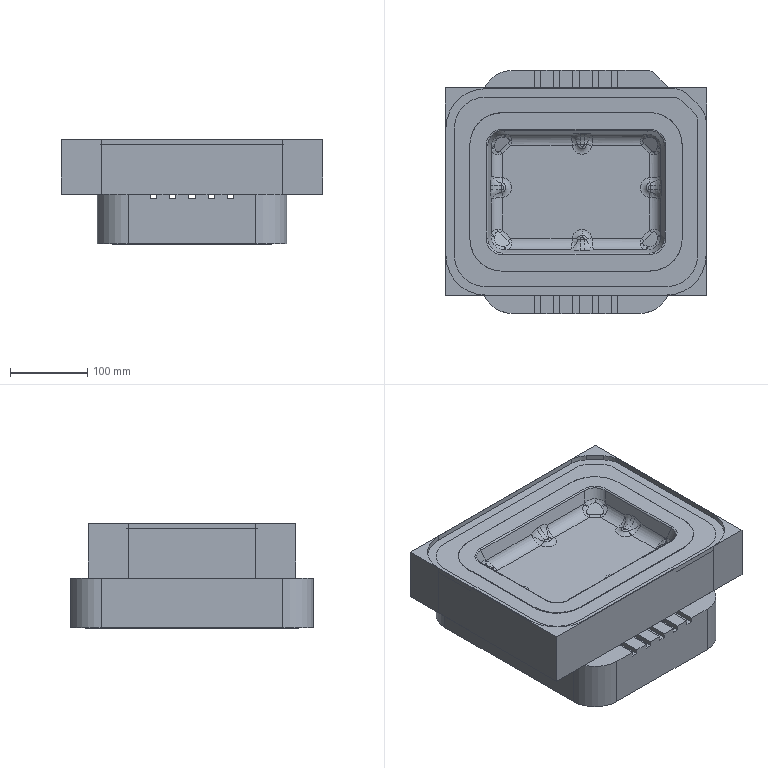NC program | NX | posted with a generic post | part box 339.125 x 315.125 x 135.5 mm
Lines 10671 to 11543 of 120728:
(B5 , TOOL : R2)
N21340 M6
N21342 G53
N21344 G17 G0 G90 X-98.635 Y-102.553 S8000 M3 M8
N21346 G43 Z220.5 H0
N21348 Z68.
N21350 G94 G1 Z65. F4500.
N21352 X-98.982 Y-102.528
N21354 X-99.175 Y-102.516
N21356 X-99.672 Y-102.466
N21358 X-100.364 Y-102.39
N21360 X-101.056 Y-102.304
N21362 X-102.004 Y-102.169
N21364 X-103.133 Y-101.974
N21366 X-103.827 Y-101.841
N21368 X-103.925 Y-101.824
N21370 X-105.484 Y-101.477
N21372 X-106.248 Y-101.281
N21374 X-106.812 Y-101.13
N21376 X-107.286 Y-100.994
N21378 X-108.324 Y-100.68
N21380 X-109.067 Y-100.437
N21382 X-109.71 Y-100.216
N21384 X-110.038 Y-100.098
N21386 X-110.051 Y-100.091
N21388 X-110.056 Y-100.087
N21390 X-110.401 Y-99.961
N21392 X-110.97 Y-99.745
N21394 X-111.095 Y-99.692
N21396 X-111.822 Y-99.401
N21398 X-112.133 Y-99.265
N21400 X-112.63 Y-99.052
N21402 G2 X-116.285 Y-97.217 R41.876
N21404 G1 X-116.711 Y-96.975
N21406 X-117.303 Y-96.627
N21408 X-118.409 Y-95.936
N21410 X-118.94 Y-95.589
N21412 X-119.449 Y-95.242
N21414 X-119.941 Y-94.896
N21416 X-120.423 Y-94.55
N21418 X-120.888 Y-94.203
N21420 X-121.342 Y-93.857
N21422 X-121.78 Y-93.511
N21424 X-122.209 Y-93.168
N21426 X-122.611 Y-92.833
N21428 X-123.035 Y-92.472
N21430 X-123.43 Y-92.125
N21432 X-123.819 Y-91.779
N21434 X-124.192 Y-91.433
N21436 X-124.581 Y-91.069
N21438 X-125.273 Y-90.394
N21440 X-125.944 Y-89.701
N21442 X-126.274 Y-89.354
N21444 X-126.593 Y-89.008
N21446 X-126.906 Y-88.662
N21448 G2 X-129.171 Y-85.891 R40.056
N21450 G1 X-129.676 Y-85.199
N21452 X-129.924 Y-84.852
N21454 X-130.161 Y-84.506
N21456 X-130.475 Y-84.046
N21458 X-130.821 Y-83.516
N21460 X-131.075 Y-83.121
N21462 X-131.707 Y-82.082
N21464 X-131.892 Y-81.756
N21466 X-132.298 Y-81.043
N21468 X-132.486 Y-80.696
N21470 X-132.549 Y-80.578
N21472 X-132.85 Y-80.004
N21474 X-133.244 Y-79.229
N21476 X-133.697 Y-78.272
N21478 X-134.283 Y-76.935
N21480 X-134.629 Y-76.08
N21482 X-134.963 Y-75.196
N21484 X-134.973 Y-75.165
N21486 X-134.975 Y-75.155
N21488 X-135.223 Y-74.462
N21490 G2 X-136.792 Y-68.575 R42.009
N21492 G1 X-136.916 Y-67.882
N21494 X-137.035 Y-67.19
N21496 X-137.138 Y-66.497
N21498 X-137.228 Y-65.804
N21500 X-137.346 Y-64.765
N21502 X-137.408 Y-64.072
N21504 X-137.499 Y-62.687
N21506 X-137.541 Y-61.648
N21508 X-137.559 Y-60.265
N21510 Y60.606
N21512 G2 X-134.845 Y75.501 R42.818
N21514 G1 X-134.581 Y76.194
N21516 X-134.304 Y76.887
N21518 X-133.939 Y77.731
N21520 X-133.853 Y77.926
N21522 X-133.59 Y78.5
N21524 X-133.535 Y78.618
N21526 X-133.2 Y79.311
N21528 X-132.898 Y79.917
N21530 X-132.671 Y80.35
N21532 X-132.552 Y80.583
N21534 X-132.102 Y81.388
N21536 X-131.86 Y81.822
N21538 X-131.511 Y82.412
N21540 X-130.821 Y83.521
N21542 X-130.398 Y84.16
N21544 X-130.129 Y84.555
N21546 X-129.437 Y85.531
N21548 X-129.427 Y85.545
N21550 X-129.369 Y85.624
N21552 X-128.912 Y86.237
N21554 G2 X-125.284 Y90.383 R42.607
N21556 G1 X-124.934 Y90.728
N21558 X-124.593 Y91.054
N21560 X-124.581 Y91.065
N21562 X-124.197 Y91.432
N21564 X-123.435 Y92.125
N21566 X-122.862 Y92.622
N21568 X-122.213 Y93.164
N21570 X-122.169 Y93.202
N21572 X-122.064 Y93.285 Z64.998
N21574 X-121.823 Y93.474 Z65.
N21576 X-121.131 Y94.019
N21578 X-120.785 Y94.278
N21580 X-120.707 Y94.337 Z64.999
N21582 X-120.425 Y94.549 Z65.
N21584 X-119.779 Y95.009
N21586 X-119.411 Y95.268
N21588 X-118.708 Y95.74
N21590 X-118.411 Y95.935
N21592 X-117.67 Y96.4
N21594 X-116.978 Y96.817
N21596 X-116.632 Y97.022
N21598 X-115.474 Y97.667
N21600 X-114.556 Y98.142
N21602 X-113.519 Y98.646
N21604 X-113.398 Y98.706
N21606 X-112.635 Y99.052
N21608 G2 X-109.018 Y100.454 R45.696
N21610 X-104.865 Y101.617 R43.031
N21612 G1 X-103.933 Y101.818
N21614 X-103.135 Y101.973
N21616 X-102.012 Y102.169
N21618 X-101.058 Y102.303
N21620 X-99.674 Y102.465
N21622 X-99.155 Y102.515
N21624 X-98.982 Y102.528
N21626 X-98.635 Y102.556
N21628 X-97.597 Y102.622
N21630 X-96.559 Y102.664
N21632 X-95.867 Y102.676
N21634 X-94.482 Y102.683
N21636 X-93.001
N21638 X95.521 Y102.68
N21640 G2 X98.284 Y102.579 R44.075
N21642 G1 X98.982 Y102.528
N21644 X99.175 Y102.516
N21646 X100.02 Y102.429
N21648 X100.712 Y102.348
N21650 X101.404 Y102.256
N21652 X102.004 Y102.169
N21654 X103.133 Y101.974
N21656 G2 X106.595 Y101.189 R38.591
N21658 G1 X106.812 Y101.13
N21660 X107.632 Y100.891
N21662 X108.324 Y100.68
N21664 X109.067 Y100.437
N21666 X109.71 Y100.216
N21668 X110.038 Y100.099
N21670 X110.051 Y100.092
N21672 X110.056 Y100.087
N21674 X110.747 Y99.831
N21676 X110.97 Y99.745
N21678 X111.095 Y99.692
N21680 X111.822 Y99.401
N21682 X112.133 Y99.265
N21684 X112.63 Y99.052
N21686 G2 X115.594 Y97.6 R42.498
N21688 G1 X116.631 Y97.023
N21690 X117.302 Y96.628
N21692 X118.409 Y95.936
N21694 X118.94 Y95.589
N21696 X119.401 Y95.275
N21698 X119.941 Y94.896
N21700 X120.423 Y94.55
N21702 X120.888 Y94.203
N21704 X121.342 Y93.857
N21706 X122.209 Y93.167
N21708 X122.611 Y92.833
N21710 X123.035 Y92.472
N21712 X123.43 Y92.125
N21714 X123.819 Y91.779
N21716 X124.58 Y91.069
N21718 X125.273 Y90.394
N21720 X125.614 Y90.047
N21722 X126.274 Y89.355
N21724 X126.593 Y89.008
N21726 X127.014 Y88.543
N21728 X127.511 Y87.969
N21730 X128.173 Y87.171 Z64.998
N21732 X128.364 Y86.93 Z65.
N21734 X128.911 Y86.238
N21736 X129.169 Y85.891
N21738 X129.226 Y85.815 Z64.999
N21740 X129.427 Y85.546 Z65.
N21742 X129.659 Y85.222
N21744 X130.156 Y84.514
N21746 X130.474 Y84.047
N21748 X130.85 Y83.474
N21750 X131.502 Y82.428
N21752 X131.909 Y81.735
N21754 X132.339 Y80.963 Z64.999
N21756 X132.486 Y80.7 Z65.
N21758 X132.552 Y80.583
N21760 X132.671 Y80.35
N21762 X132.898 Y79.917
N21764 G2 X134.295 Y76.897 R41.824
N21766 G1 X134.439 Y76.54
N21768 X134.714 Y75.848
N21770 G2 X136.855 Y68.228 R42.18
N21772 G1 X137.035 Y67.19
N21774 X137.089 Y66.843
N21776 X137.185 Y66.15
N21778 X137.346 Y64.765
N21780 X137.377 Y64.432
N21782 X137.397 Y64.225
N21784 X137.434 Y63.726
N21786 X137.499 Y62.687
N21788 X137.541 Y61.648
N21790 X137.558 Y60.609
N21792 X137.556 Y-60.609
N21794 X137.551 Y-60.949
N21796 X137.53 Y-61.988
N21798 X137.5 Y-62.687
N21800 X137.461 Y-63.374
N21802 X137.397 Y-64.239
N21804 X137.272 Y-65.456
N21806 X137.186 Y-66.148
N21808 X137.051 Y-67.097
N21810 X136.916 Y-67.882
N21812 X136.792 Y-68.575
N21814 G2 X135.455 Y-73.766 R40.941
N21816 G1 X135.322 Y-74.166
N21818 X134.975 Y-75.155
N21820 X134.629 Y-76.075
N21822 X134.304 Y-76.886
N21824 X134.153 Y-77.233
N21826 X133.853 Y-77.926
N21828 X133.695 Y-78.272
N21830 X133.59 Y-78.505
N21832 X133.244 Y-79.224
N21834 X132.898 Y-79.917
N21836 X132.851 Y-80.004
N21838 X132.552 Y-80.582
N21840 X132.542 Y-80.6
N21842 X131.909 Y-81.735
N21844 X131.508 Y-82.417
N21846 X131.07 Y-83.121
N21848 X130.932 Y-83.342 Z64.998
N21850 X130.855 Y-83.467 Z65.
N21852 X130.475 Y-84.046
N21854 X130.398 Y-84.16
N21856 X130.243 Y-84.387 Z64.998
N21858 X130.162 Y-84.506 Z65.
N21860 X129.437 Y-85.534
N21862 X128.912 Y-86.237
N21864 X128.398 Y-86.887
N21866 X128.173 Y-87.171 Z64.998
N21868 X128.091 Y-87.276 Z65.
N21870 X127.512 Y-87.969
N21872 X127.209 Y-88.316
N21874 X126.668 Y-88.927
N21876 X125.976 Y-89.674
N21878 X125.293 Y-90.374
N21880 X124.938 Y-90.724
N21882 X124.196 Y-91.433
N21884 X123.435 Y-92.125
N21886 X122.862 Y-92.622
N21888 X122.214 Y-93.164
N21890 X122.169 Y-93.202
N21892 X121.341 Y-93.857
N21894 X120.439 Y-94.538
N21896 X119.403 Y-95.273
N21898 X118.362 Y-95.963
N21900 X117.324 Y-96.611
N21902 X116.632 Y-97.022
N21904 X115.474 Y-97.667
N21906 X114.556 Y-98.142
N21908 X113.398 Y-98.706
N21910 X112.635 Y-99.052
N21912 X112.479 Y-99.117
N21914 G2 X109.364 Y-100.335 R40.751
N21916 G1 X108.672 Y-100.567
N21918 X107.998 Y-100.783
N21920 X107.288 Y-100.994
N21922 X106.595 Y-101.189
N21924 X105.742 Y-101.411
N21926 X105.557 Y-101.458
N21928 X105.487 Y-101.475
N21930 X104.173 Y-101.77
N21932 X103.931 Y-101.82
N21934 X103.869 Y-101.832
N21936 X103.135 Y-101.973
N21938 X102.012 Y-102.169
N21940 X101.058 Y-102.303
N21942 X100.02 Y-102.428
N21944 X99.155 Y-102.514
N21946 X98.635 Y-102.556
N21948 X97.597 Y-102.622
N21950 X96.559 Y-102.664
N21952 X95.521 Y-102.677
N21954 X93.344 Y-102.682
N21956 X-95.518
N21958 X-96.899 Y-102.654
N21960 X-97.251 Y-102.64
N21962 X-97.943 Y-102.602
N21964 X-98.635 Y-102.553
N21966 X-98.633 Y-102.515
N21968 Y-102.513
N21970 X-98.615 Y-102.269
N21972 G2 X-116.89 Y-96.539 R42.14
N21974 G1 X-117.102 Y-96.414
N21976 X-117.318 Y-96.281
N21978 X-117.765 Y-96.003
N21980 G2 X-121.193 Y-93.612 R37.448
N21982 G1 X-121.986 Y-92.98
N21984 X-122.862 Y-92.244
N21986 X-123.645 Y-91.551
N21988 X-124.008 Y-91.215
N21990 X-124.145 Y-91.086
N21992 X-124.369 Y-90.876
N21994 X-124.51 Y-90.74
N21996 X-125.075 Y-90.189
N21998 X-125.752 Y-89.489
N22000 X-126.087 Y-89.137
N22002 X-126.669 Y-88.499
N22004 G2 X-129.437 Y-85.042 R40.433
N22006 G1 X-129.504 Y-84.949
N22008 X-129.66 Y-84.729
N22010 G2 X-136.627 Y-67.882 R41.805
N22012 G1 X-136.746 Y-67.189
N22014 X-136.789 Y-66.905
N22016 G2 X-137.273 Y-60.485 R42.688
N22018 G1 X-137.271 Y60.735
N22020 G2 X-136.79 Y66.905 R43.353
N22022 G1 X-136.748 Y67.178
N22024 X-136.61 Y67.977
N22026 G2 X-126.441 Y88.752 R41.672
N22028 G1 X-125.63 Y89.62
N22030 X-125.079 Y90.184
N22032 X-124.732 Y90.527
N22034 X-124.011 Y91.216
N22036 X-123.276 Y91.884
N22038 X-123.208 Y91.944
N22040 X-122.903 Y92.209
N22042 X-122.597 Y92.472
N22044 G2 X-120.439 Y94.182 R43.174
N22046 G1 X-119.842 Y94.614
N22048 G2 X-102.884 Y101.727 R41.737
N22050 G1 X-102.096 Y101.865
N22052 X-101.814 Y101.908
N22054 G2 X-94.482 Y102.398 R44.723
N22056 G1 X-92.999
N22058 X95.745 Y102.393
N22060 G2 X116.632 Y96.691 R42.242
N22062 G1 X117.102 Y96.414
N22064 X117.318 Y96.281
N22066 X117.765 Y96.003
N22068 G2 X121.193 Y93.612 R37.404
N22070 G1 X121.986 Y92.98
N22072 G2 X125.881 Y89.355 R41.06
N22074 G1 X126.09 Y89.134
N22076 X126.415 Y88.78
N22078 X126.773 Y88.384
N22080 X127.361 Y87.705
N22082 X128. Y86.93
N22084 X128.468 Y86.338
N22086 X128.635 Y86.127
N22088 G2 X132.882 Y79.311 R41.713
N22090 G1 X133.011 Y79.047
N22092 X133.244 Y78.567
N22094 G2 X136.587 Y68.109 R42.183
N22096 G1 X136.746 Y67.189
N22098 X136.791 Y66.906
N22100 X136.914 Y66.013
N22102 X137.058 Y64.774
N22104 X137.088 Y64.461
N22106 X137.12 Y64.102
N22108 X137.213 Y62.687
N22110 X137.258 Y61.508
N22112 X137.273 Y60.485
N22114 X137.271 Y-60.736
N22116 G2 X136.79 Y-66.905 R42.125
N22118 G1 X136.748 Y-67.178
N22120 X136.626 Y-67.882
N22122 G2 X124.732 Y-90.527 R41.649
N22124 G1 X124.019 Y-91.208
N22126 X123.9 Y-91.317
N22128 X123.276 Y-91.884
N22130 X123.208 Y-91.944
N22132 X122.903 Y-92.209
N22134 X122.597 Y-92.472
N22136 X122.098 Y-92.89
N22138 X121.823 Y-93.112
N22140 X121.219 Y-93.59
N22142 X121.131 Y-93.659
N22144 X120.439 Y-94.181
N22146 X119.935 Y-94.55
N22148 X119.294 Y-95.003
N22150 X119.055 Y-95.164
N22152 X118.816 Y-95.324
N22154 X118.256 Y-95.695
N22156 G2 X112.825 Y-98.653 R41.36
N22158 G1 X112.518 Y-98.792
N22160 X112.301 Y-98.884
N22162 G2 X102.884 Y-101.727 R42.181
N22164 G1 X102.096 Y-101.865
N22166 X101.814 Y-101.908
N22168 G2 X94.947 Y-102.397 R43.692
N22170 G1 X-95.521 Y-102.396
N22172 X-97.096 Y-102.361
N22174 X-97.943 Y-102.316
N22176 X-98.289 Y-102.292
N22178 X-98.615 Y-102.269
N22180 X-98.595 Y-101.985
N22182 G2 X-131.962 Y-80.467 R41.314
N22184 X-136.988 Y-60.546 R42.052
N22186 G1 X-136.987 Y60.673
N22188 G2 X-122.862 Y91.867 R41.557
N22190 X-95.582 Y102.108 R41.692
N22192 G1 X-94.539 Y102.113
N22194 X-93.054
N22196 X95.521 Y102.111
N22198 G2 X126.669 Y88.071 R41.574
N22200 X136.988 Y60.546 R41.746
N22202 G1 X136.987 Y-60.673
N22204 G2 X122.169 Y-92.458 R41.534
N22206 X94.886 Y-102.112 R41.766
N22208 G1 X-95.521 Y-102.111
N22210 X-96.905 Y-102.082
N22212 X-97.943 Y-102.03
N22214 X-98.137 Y-102.017
N22216 X-98.595 Y-101.985
N22218 X-98.574 Y-101.7
N22220 G2 X-129.783 Y-83.541 R41.056
N22222 X-136.703 Y-60.609 R41.644
N22224 G1 Y60.609
N22226 G2 X-126.066 Y88.316 R41.437
N22228 X-95.868 Y101.821 R41.265
N22230 G1 X-94.483 Y101.828
N22232 X-92.999
N22234 X95.52 Y101.827
N22236 G2 X123.973 Y90.467 R41.345
N22238 X136.703 Y60.609 R41.317
N22240 G1 Y-60.609
N22242 G2 X121.477 Y-92.658 R41.246
N22244 X95.175 Y-101.827 R41.47
N22246 G1 X-95.52
N22248 G2 X-98.574 Y-101.7 R40.082
N22250 G1 X-98.554 Y-101.416
N22252 G2 X-132.206 Y-78.753 R40.754
N22254 X-136.418 Y-60.609 R41.562
N22256 G1 Y60.609
N22258 G2 X-121.677 Y92.125 R40.977
N22260 X-95.867 Y101.536 R41.103
N22262 G1 X-94.482 Y101.543
N22264 X-92.998
N22266 X95.521 Y101.542
N22268 G2 X124.816 Y89.232 R41.04
N22270 X136.418 Y60.609 R41.136
N22272 G1 Y-60.609
N22274 G2 X120.439 Y-93.11 R40.95
N22276 X95.175 Y-101.542 R41.242
N22278 G1 X-95.521
N22280 G2 X-98.554 Y-101.416 R39.818
N22282 G1 X-98.533 Y-101.131
N22284 G2 X-131.168 Y-80.139 R40.473
N22286 X-136.133 Y-60.609 R41.189
N22288 G1 Y60.609
N22290 G2 X-123.217 Y90.394 R40.739
N22292 X-95.867 Y101.251 R40.826
N22294 G1 X-94.482 Y101.258
N22296 X-92.998
N22298 X95.521 Y101.257
N22300 G2 X124.603 Y89.043 R40.756
N22302 X136.133 Y60.609 R40.812
N22304 G1 Y-60.609
N22306 G2 X121.131 Y-92.204 R40.682
N22308 X95.175 Y-101.257 R40.968
N22310 G1 X-95.521
N22312 G2 X-98.533 Y-101.131 R39.719
N22314 G1 X-98.513 Y-100.847
N22316 G2 X-127.913 Y-84.713 R40.237
N22318 X-135.848 Y-60.444 R40.715
N22320 G1 X-135.846 Y60.776
N22322 G2 X-123.554 Y89.681 R40.421
N22324 X-95.683 Y100.967 R40.479
N22326 G1 X-94.482 Y100.973
N22328 X-92.999
N22330 X95.705 Y100.969
N22332 G2 X125.738 Y87.403 R40.426
N22334 X135.848 Y60.444 R40.599
N22336 G1 X135.844 Y-60.778
N22338 G2 X122.169 Y-90.956 R40.393
N22340 X94.987 Y-100.972 R40.656
N22342 G1 X-95.521 Y-100.971
N22344 X-97.057 Y-100.935
N22346 X-98.04 Y-100.881
N22348 X-98.513 Y-100.847
N22350 X-98.492 Y-100.563
N22352 G2 X-128.844 Y-82.892 R39.925
N22354 X-135.563 Y-60.609 R40.493
N22356 G1 Y60.609
N22358 G2 X-121.172 Y91.433 R40.151
N22360 X-95.867 Y100.681 R40.305
N22362 G1 X-94.482 Y100.688
N22364 X-92.998
N22366 X95.521 Y100.687
N22368 G2 X126.184 Y86.446 R40.151
N22370 X135.563 Y60.609 R40.371
N22372 G1 Y-60.609
N22374 G2 X123.832 Y-89.008 R40.28
N22376 X95.175 Y-100.687 R40.246
N22378 G1 X-95.521
N22380 G2 X-98.492 Y-100.563 R39.978
N22382 G1 X-98.472 Y-100.278
N22384 G2 X-128.745 Y-82.524 R39.638
N22386 X-135.278 Y-60.609 R40.276
N22388 G1 Y60.609
N22390 G2 X-123.774 Y88.662 R40.016
N22392 X-95.867 Y100.396 R39.94
N22394 G1 X-94.517 Y100.403
N22396 X-93.032
N22398 X95.521 Y100.402
N22400 G2 X123.141 Y89.288 R40.029
N22402 X135.278 Y60.609 R39.9
N22404 G1 Y-60.609
N22406 G2 X121.477 Y-90.801 R39.898
N22408 X95.175 Y-100.402 R40.018
N22410 G1 X-95.521
N22412 G2 X-98.472 Y-100.278 R39.661
N22414 G1 X-98.452 Y-99.994
N22416 G2 X-129.543 Y-80.696 R39.341
N22418 X-134.993 Y-60.609 R40.046
N22420 G1 Y60.588
N22422 G2 X-119.474 Y92.052 R39.522
N22424 X-94.485 Y100.118 R39.955
N22426 G1 X-93.001
N22428 X95.518 Y100.117
N22430 G2 X125.141 Y86.787 R39.624
N22432 X134.993 Y60.609 R39.752
N22434 G1 Y-60.609
N22436 G2 X121.131 Y-90.721 R39.577
N22438 X95.178 Y-100.117 R39.8
N22440 G1 X-95.518
N22442 G2 X-98.452 Y-99.994 R39.354
N22444 G1 X-98.431 Y-99.71
N22446 G2 X-127.015 Y-84.01 R39.072
N22448 X-134.708 Y-60.609 R39.591
N22450 G1 Y60.609
N22452 G2 X-120.439 Y90.928 R39.277
N22454 X-94.482 Y99.833 R39.661
N22456 G1 X-92.998
N22458 X95.521 Y99.831
N22460 G2 X124.266 Y87.328 R39.333
N22462 X134.708 Y60.609 R39.432
N22464 G1 Y-60.609
N22466 G2 X121.077 Y-90.394 R39.295
N22468 X95.175 Y-99.832 R39.5
N22470 G1 X-95.521 Y-99.831
N22472 G2 X-98.431 Y-99.71 R39.062
N22474 G1 X-98.411 Y-99.425
N22476 G2 X-128.425 Y-81.44 R38.788
N22478 X-134.423 Y-60.403 R39.448
N22480 G1 X-134.422 Y60.609
N22482 G2 X-123.554 Y87.663 R39.165
N22484 X-95.724 Y99.542 R39.039
N22486 G1 X-94.482 Y99.548
N22488 X-93.001
N22490 X95.666 Y99.544
N22492 G2 X125.842 Y85.064 R38.993
N22494 X134.423 Y60.403 R39.216
N22496 G1 X134.422 Y-60.609
N22498 G2 X122.555 Y-88.662 R39.116
N22500 X95.026 Y-99.547 R39.136
N22502 G1 X-95.665 Y-99.543
N22504 X-97.017 Y-99.51
N22506 X-97.943 Y-99.459
N22508 X-98.411 Y-99.425
N22510 X-98.39 Y-99.141
N22512 G2 X-126.544 Y-83.688 R38.516
N22514 X-134.138 Y-60.609 R39.064
N22516 G1 Y60.609
N22518 G2 X-118.016 Y92.063 R38.662
N22520 X-94.482 Y99.263 R39.173
N22522 G1 X-92.998
N22524 X95.521 Y99.261
N22526 G2 X123.529 Y87.277 R38.766
N22528 X134.138 Y60.609 R38.889
N22530 G1 X134.137 Y-60.609
N22532 G2 X118.234 Y-91.907 R38.68
N22534 X95.175 Y-99.262 R39.016
N22536 G1 X-95.521 Y-99.261
N22538 G2 X-98.39 Y-99.141 R38.333
N22540 G1 X-98.369 Y-98.857
N22542 G2 X-129.159 Y-79.057 R38.206
N22544 X-133.853 Y-60.609 R39.
N22546 G1 Y60.609
N22548 G2 X-122.448 Y87.969 R38.563
N22550 X-95.867 Y98.971 R38.504
N22552 G1 X-94.482 Y98.978
N22554 X-92.998
N22556 X95.521 Y98.976
N22558 G2 X124.318 Y85.996 R38.5
N22560 X133.853 Y60.609 R38.685
N22562 G1 X133.852 Y-60.609
N22564 G2 X119.055 Y-90.936 R38.406
N22566 X95.175 Y-98.977 R38.673
N22568 G1 X-95.521 Y-98.976
N22570 G2 X-98.369 Y-98.857 R38.016
N22572 G1 X-98.348 Y-98.572
N22574 G2 X-125.84 Y-83.677 R37.959
N22576 X-133.568 Y-60.609 R38.45
N22578 G1 Y60.609
N22580 G2 X-122.392 Y87.623 R38.28
N22582 X-95.867 Y98.686 R38.216
N22584 G1 X-94.495 Y98.693
N22586 X-93.011
N22588 X95.506 Y98.691
N22590 G2 X124.131 Y85.776 R38.207
N22592 X133.568 Y60.609 R38.347
N22594 G1 X133.567 Y-60.609
N22596 G2 X122.392 Y-87.623 R38.277
N22598 X95.189 Y-98.691 R38.28
N22600 G1 X-95.506
N22602 G2 X-98.348 Y-98.572 R37.7
N22604 G1 X-98.327 Y-98.288
N22606 G2 X-126.51 Y-82.269 R37.664
N22608 X-133.283 Y-60.609 R38.22
N22610 G1 Y60.609
N22612 G2 X-116.632 Y91.982 R37.792
N22614 X-95.869 Y98.401 R38.166
N22616 G1 X-94.484 Y98.408
N22618 X-93.
N22620 X95.519 Y98.406
N22622 G2 X124.089 Y85.388 R37.893
N22624 X133.283 Y60.609 R38.056
N22626 G1 X133.282 Y-60.609
N22628 G2 X118.823 Y-90.394 R37.817
N22630 X95.177 Y-98.406 R38.112
N22632 G1 X-95.519
N22634 G2 X-98.327 Y-98.288 R37.13
N22636 G1 X-98.307 Y-98.003
N22638 G2 X-126.862 Y-81.236 R37.374
N22640 X-132.997 Y-60.609 R37.965
N22642 G1 Y60.609
N22644 G2 X-122.862 Y86.319 R37.771
N22646 X-95.764 Y98.116 R37.629
N22648 G1 X-94.482 Y98.123
N22650 X-93.001
N22652 X95.627 Y98.119
N22654 G2 X123.726 Y85.371 R37.607
N22656 X132.998 Y60.362 R37.773
N22658 G1 X132.997 Y-60.609
N22660 G2 X120.785 Y-88.366 R37.664
N22662 X95.066 Y-98.121 R37.742
N22664 G1 X-95.626 Y-98.119
N22666 X-96.971 Y-98.086
N22668 X-97.941 Y-98.03
N22670 X-98.307 Y-98.003
N22672 X-98.286 Y-97.719
N22674 G2 X-124.924 Y-83.467 R37.118
N22676 X-132.712 Y-60.609 R37.628
N22678 G1 X-132.713 Y60.609
N22680 G2 X-121.477 Y87.322 R37.415
N22682 X-95.867 Y97.831 R37.376
N22684 G1 X-94.482 Y97.838
N22686 X-92.998
N22688 X95.521 Y97.836
N22690 G2 X119.692 Y88.953 R37.593
N22692 X132.691 Y61.648 R37.24
N22694 G1 X132.712 Y60.609
N22696 Y-60.609
N22698 G2 X117.095 Y-90.97 R37.253
N22700 X95.175 Y-97.836 R37.601
N22702 G1 X-95.521
N22704 X-96.559 Y-97.813
N22706 X-96.905 Y-97.804
N22708 X-97.993 Y-97.741
N22710 X-98.286 Y-97.719
N22712 X-98.264 Y-97.435
N22714 G2 X-125.284 Y-82.512 R36.809
N22716 X-132.427 Y-60.484 R37.256
N22718 G1 X-132.425 Y60.736
N22720 G2 X-118.317 Y89.701 R36.947
N22722 X-95.641 Y97.547 R37.18
N22724 G1 X-94.482 Y97.553
N22726 X-92.999 Y97.552
N22728 X95.521 Y97.55
N22730 G2 X123.161 Y85.152 R37.059
N22732 X132.427 Y60.484 R37.199
N22734 G1 X132.424 Y-60.737
N22736 G2 X117.404 Y-90.394 R36.944
N22738 X94.944 Y-97.551 R37.303
N22740 G1 X-95.521 Y-97.55
N22742 X-96.905 Y-97.518
N22744 X-98.072 Y-97.449
N22746 X-98.264 Y-97.435
N22748 X-98.243 Y-97.15
N22750 G2 X-124.66 Y-82.873 R36.524
N22752 X-132.142 Y-60.609 R36.951
N22754 G1 Y60.609
N22756 G2 X-117.392 Y90.047 R36.693
N22758 X-95.867 Y97.26 R36.961
N22760 G1 X-94.535 Y97.267
N22762 X-93.051
N22764 X95.521 Y97.266
N22766 G2 X123.121 Y84.765 R36.764
N22768 X132.142 Y60.609 R36.922
N22770 G1 Y-60.609
N22772 G2 X116.632 Y-90.598 R36.683
N22774 X95.175 Y-97.266 R37.014
N22776 G1 X-95.521
N22778 X-96.559 Y-97.243
N22780 X-96.905 Y-97.233
N22782 X-97.943 Y-97.173
N22784 X-98.243 Y-97.15
N22786 X-98.222 Y-96.866
N22788 G2 X-125.384 Y-81.389 R36.232
N22790 X-131.857 Y-60.609 R36.82
N22792 G1 Y60.609
N22794 G2 X-121.355 Y86.238 R36.577
N22796 X-95.867 Y96.975 R36.526
N22798 G1 X-94.484 Y96.982
N22800 X-92.999
N22802 X95.519 Y96.981
N22804 G2 X122.577 Y84.949 R36.488
N22806 X131.857 Y60.609 R36.632
N22808 G1 Y-60.609
N22810 G2 X116.427 Y-90.394 R36.392
N22812 X95.176 Y-96.981 R36.742
N22814 G1 X-95.519
N22816 X-96.543 Y-96.958
N22818 X-96.879 Y-96.948
N22820 X-97.943 Y-96.887
N22822 X-98.222 Y-96.866
N22824 X-98.2 Y-96.582
N22826 G2 X-124.246 Y-82.475 R35.962
N22828 X-131.572 Y-60.609 R36.408
N22830 G1 Y60.609
N22832 G2 X-121.63 Y85.545 R36.317
N22834 X-95.867 Y96.69 R36.206
N22836 G1 X-94.482 Y96.697
N22838 X-92.998
N22840 X95.521 Y96.696
N22842 G2 X122.169 Y84.973 R36.203
N22844 X131.572 Y60.609 R36.329
N22846 G1 Y-60.609
N22848 G2 X118.362 Y-88.571 R36.15
N22850 X95.175 Y-96.696 R36.378
N22852 G1 X-95.521 Y-96.695
N22854 X-96.557 Y-96.673
N22856 X-96.902 Y-96.662
N22858 X-97.918 Y-96.603
N22860 X-98.2 Y-96.582
N22862 X-98.179 Y-96.297
N22864 G2 X-126.402 Y-78.721 R35.634
N22866 X-131.287 Y-60.609 R36.306
N22868 G1 Y60.609
N22870 G2 X-120.895 Y85.891 R36.019
N22872 X-95.867 Y96.405 R35.933
N22874 G1 X-94.482 Y96.412
N22876 X95.521 Y96.411
N22878 G2 X121.477 Y85.297 R35.925
N22880 X131.287 Y60.609 R36.019
N22882 G1 Y-60.609
N22884 G2 X118.016 Y-88.485 R35.865
N22886 X95.175 Y-96.411 R36.112
N22888 G1 X-95.521 Y-96.41
N22890 X-96.559 Y-96.388
N22892 X-96.905 Y-96.377
N22894 X-97.941 Y-96.315
N22896 X-98.179 Y-96.297
N22898 X-98.157 Y-96.013
N22900 G2 X-123.859 Y-82.041 R35.375
N22902 X-131.002 Y-60.443 R35.861
N22904 G1 X-130.999 Y60.777
N22906 G2 X-120.093 Y86.278 R35.692
N22908 X-95.681 Y96.121 R35.643
N22910 G1 X-94.482 Y96.127
N22912 X-92.999
N22914 X95.708 Y96.122
N22916 G2 X120.785 Y85.607 R35.628
N22918 X131.002 Y60.443 R35.727
N22920 G1 X131.001 Y-60.609
N22922 G2 X117.331 Y-88.662 R35.563
N22924 X94.984 Y-96.126 R35.804
N22926 G1 X-95.521 Y-96.125
N22928 X-96.905 Y-96.091
N22930 X-97.943 Y-96.029
N22932 X-98.157 Y-96.013
N22934 X-98.136 Y-95.729
N22936 G2 X-123.471 Y-82.082 R35.125
N22938 X-130.717 Y-60.609 R35.569
N22940 G1 Y60.609
N22942 G2 X-117.67 Y88.03 R35.29
N22944 X-95.867 Y95.835 R35.458
N22946 G1 X-94.482 Y95.842
N22948 X95.521 Y95.841
N22950 G2 X120.785 Y85.199 R35.381
N22952 X130.717 Y60.609 R35.444
N22954 G1 Y-60.609
N22956 G2 X118.016 Y-87.748 R35.296
N22958 X95.175 Y-95.841 R35.517
N22960 G1 X-95.521 Y-95.84
N22962 X-96.559 Y-95.817
N22964 X-96.905 Y-95.806
N22966 X-97.943 Y-95.744
N22968 X-98.136 Y-95.729
N22970 X-98.143 Y-95.443
N22972 G2 X-123.633 Y-81.389 R34.814
N22974 X-130.432 Y-60.565 R35.324
N22976 G1 X-130.431 Y60.653
N22978 G2 X-120.375 Y85.199 R35.162
N22980 X-95.867 Y95.55 R35.077
N22982 G1 X-94.514 Y95.557
N22984 X95.521 Y95.555
N22986 G2 X120.387 Y85.199 R35.109
N22988 X130.432 Y60.565 R35.115
N22990 G1 X130.431 Y-60.654
N22992 G2 X116.286 Y-88.737 R34.982
N22994 X95.175 Y-95.556 R35.272
N22996 G1 X-95.521 Y-95.555
N22998 X-96.905 Y-95.52
N23000 X-97.943 Y-95.458
N23002 X-98.143 Y-95.443
N23004 X-98.122 Y-95.158
N23006 G2 X-122.476 Y-82.428 R34.573
N23008 X-130.147 Y-60.609 R34.932
N23010 G1 Y60.591
N23012 G2 X-117.266 Y87.623 R34.737
N23014 X-95.87 Y95.265 R34.911
N23016 G1 X-94.485 Y95.272
N23018 X95.518 Y95.271
N23020 G2 X120.719 Y84.44 R34.789
N23022 X130.147 Y60.609 R34.905
N23024 G1 X130.146 Y-60.609
N23026 G2 X116.374 Y-88.316 R34.704
N23028 X95.178 Y-95.271 R34.974
N23030 G1 X-95.518 Y-95.27
N23032 X-96.558 Y-95.247
N23034 X-96.898 Y-95.235
N23036 X-97.943 Y-95.172
N23038 X-98.122 Y-95.158
N23040 X-98.1 Y-94.874
N23042 G2 X-123.43 Y-80.696 R34.242
N23044 X-129.862 Y-60.609 R34.684
N23046 G1 Y60.609
N23048 G2 X-119.915 Y84.852 R34.585
N23050 X-95.867 Y94.98 R34.505
N23052 G1 X-94.482 Y94.987
N23054 X95.521 Y94.986
N23056 G2 X119.839 Y84.944 R34.573
N23058 X129.862 Y60.609 R34.599
N23060 G1 X129.861 Y-60.609
N23062 G2 X117.241 Y-87.277 R34.441
N23064 X95.175 Y-94.986 R34.634
N23066 G1 X-95.521 Y-94.985
N23068 X-96.559 Y-94.962
N23070 X-96.904 Y-94.95
N23072 X-98.1 Y-94.874
N23074 X-98.078 Y-94.59
N23076 G2 X-124.032 Y-79.311 R33.944
N23078 X-129.577 Y-60.402 R34.61